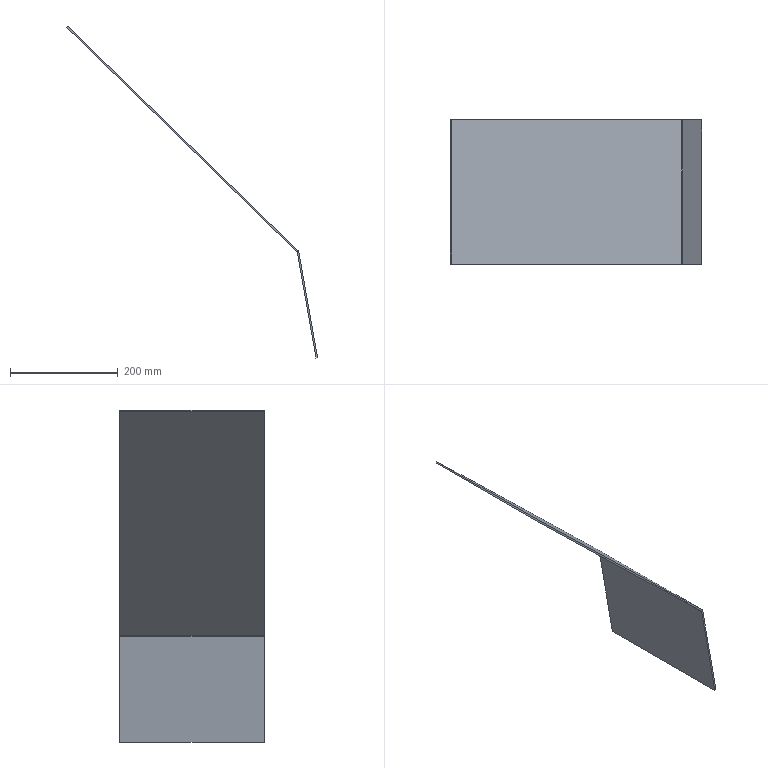Part | STEP file | floating channel bottom plate--2025.12.03 | 1 solid | 10 faces | box 466.015 x 268.5 x 616.159 mm | volume 643321 mm3 | plane 8 | cylinder 2 | commonest cylinder face diameters 6 x1 12 x1
STEP:
#1=CARTESIAN_POINT('',(0.,0.,0.));
#2=DIRECTION('',(0.,0.,1.));
#3=DIRECTION('',(1.,0.,0.));
#4=AXIS2_PLACEMENT_3D('',#1,#2,#3);
#5=CARTESIAN_POINT('',(1644.219,36.5,96.));
#6=VERTEX_POINT('',#5);
#7=CARTESIAN_POINT('',(2071.793,36.5,-320.384));
#8=VERTEX_POINT('',#7);
#9=CARTESIAN_POINT('',(1644.219,36.5,96.));
#10=DIRECTION('',(0.7164,0.,-0.6977));
#11=VECTOR('',#10,1.);
#12=LINE('',#9,#11);
#13=CARTESIAN_POINT('',(1644.219,305.,96.));
#14=DIRECTION('',(-0.6977,0.,-0.7164));
#15=DIRECTION('',(0.7164,0.,-0.6977));
#16=AXIS2_PLACEMENT_3D('',#13,#14,#15);
#17=PLANE('',#16);
#18=CARTESIAN_POINT('',(0.,268.5));
#19=DIRECTION('',(1.,0.));
#20=VECTOR('',#19,1.);
#21=LINE('',#18,#20);
#22=(GEOMETRIC_REPRESENTATION_CONTEXT(2)PARAMETRIC_REPRESENTATION_CONTEXT()REPRESENTATION_CONTEXT('',''));
#23=DEFINITIONAL_REPRESENTATION('',(#21),#22);
#24=PCURVE('',#17,#23);
#25=CARTESIAN_POINT('',(0.,36.5,0.));
#26=DIRECTION('',(0.,-1.,0.));
#27=DIRECTION('',(0.,0.,1.));
#28=AXIS2_PLACEMENT_3D('',#25,#26,#27);
#29=PLANE('',#28);
#30=CARTESIAN_POINT('',(96.,-1644.219));
#31=DIRECTION('',(-0.6977,-0.7164));
#32=VECTOR('',#31,1.);
#33=LINE('',#30,#32);
#34=(GEOMETRIC_REPRESENTATION_CONTEXT(2)PARAMETRIC_REPRESENTATION_CONTEXT()REPRESENTATION_CONTEXT('',''));
#35=DEFINITIONAL_REPRESENTATION('',(#33),#34);
#36=PCURVE('',#29,#35);
#37=SURFACE_CURVE('',#12,(#24,#36),.PCURVE_S1.);
#38=EDGE_CURVE('',#6,#8,#37,.T.);
#39=ORIENTED_EDGE('',*,*,#38,.T.);
#40=CARTESIAN_POINT('',(2071.793,305.,-320.384));
#41=VERTEX_POINT('',#40);
#42=CARTESIAN_POINT('',(2071.793,305.,-320.384));
#43=DIRECTION('',(0.,1.,0.));
#44=VECTOR('',#43,1.);
#45=LINE('',#42,#44);
#46=CARTESIAN_POINT('',(596.821,0.));
#47=DIRECTION('',(0.,-1.));
#48=VECTOR('',#47,1.);
#49=LINE('',#46,#48);
#50=(GEOMETRIC_REPRESENTATION_CONTEXT(2)PARAMETRIC_REPRESENTATION_CONTEXT()REPRESENTATION_CONTEXT('',''));
#51=DEFINITIONAL_REPRESENTATION('',(#49),#50);
#52=PCURVE('',#17,#51);
#53=CARTESIAN_POINT('',(2067.606,305.,-324.683));
#54=DIRECTION('',(0.,-1.,0.));
#55=DIRECTION('',(0.,0.,1.));
#56=AXIS2_PLACEMENT_3D('',#53,#54,#55);
#57=CYLINDRICAL_SURFACE('',#56,6.);
#58=CARTESIAN_POINT('',(5.511,0.));
#59=DIRECTION('',(0.,-1.));
#60=VECTOR('',#59,1.);
#61=LINE('',#58,#60);
#62=(GEOMETRIC_REPRESENTATION_CONTEXT(2)PARAMETRIC_REPRESENTATION_CONTEXT()REPRESENTATION_CONTEXT('',''));
#63=DEFINITIONAL_REPRESENTATION('',(#61),#62);
#64=PCURVE('',#57,#63);
#65=SURFACE_CURVE('',#45,(#52,#64),.PCURVE_S1.);
#66=EDGE_CURVE('',#8,#41,#65,.T.);
#67=ORIENTED_EDGE('',*,*,#66,.T.);
#68=CARTESIAN_POINT('',(1644.219,305.,96.));
#69=VERTEX_POINT('',#68);
#70=CARTESIAN_POINT('',(1644.219,305.,96.));
#71=DIRECTION('',(0.7164,0.,-0.6977));
#72=VECTOR('',#71,1.);
#73=LINE('',#70,#72);
#74=CARTESIAN_POINT('',(0.,0.));
#75=DIRECTION('',(1.,0.));
#76=VECTOR('',#75,1.);
#77=LINE('',#74,#76);
#78=(GEOMETRIC_REPRESENTATION_CONTEXT(2)PARAMETRIC_REPRESENTATION_CONTEXT()REPRESENTATION_CONTEXT('',''));
#79=DEFINITIONAL_REPRESENTATION('',(#77),#78);
#80=PCURVE('',#17,#79);
#81=CARTESIAN_POINT('',(0.,305.,0.));
#82=DIRECTION('',(0.,-1.,0.));
#83=DIRECTION('',(0.,0.,1.));
#84=AXIS2_PLACEMENT_3D('',#81,#82,#83);
#85=PLANE('',#84);
#86=CARTESIAN_POINT('',(96.,-1644.219));
#87=DIRECTION('',(-0.6977,-0.7164));
#88=VECTOR('',#87,1.);
#89=LINE('',#86,#88);
#90=(GEOMETRIC_REPRESENTATION_CONTEXT(2)PARAMETRIC_REPRESENTATION_CONTEXT()REPRESENTATION_CONTEXT('',''));
#91=DEFINITIONAL_REPRESENTATION('',(#89),#90);
#92=PCURVE('',#85,#91);
#93=SURFACE_CURVE('',#73,(#80,#92),.PCURVE_S1.);
#94=EDGE_CURVE('',#69,#41,#93,.T.);
#95=ORIENTED_EDGE('',*,*,#94,.F.);
#96=CARTESIAN_POINT('',(1644.219,305.,96.));
#97=DIRECTION('',(0.,-1.,0.));
#98=VECTOR('',#97,1.);
#99=LINE('',#96,#98);
#100=CARTESIAN_POINT('',(0.,0.));
#101=DIRECTION('',(0.,1.));
#102=VECTOR('',#101,1.);
#103=LINE('',#100,#102);
#104=(GEOMETRIC_REPRESENTATION_CONTEXT(2)PARAMETRIC_REPRESENTATION_CONTEXT()REPRESENTATION_CONTEXT('',''));
#105=DEFINITIONAL_REPRESENTATION('',(#103),#104);
#106=PCURVE('',#17,#105);
#107=CARTESIAN_POINT('',(1642.126,305.,93.851));
#108=DIRECTION('',(0.7164,0.,-0.6977));
#109=DIRECTION('',(0.6977,0.,0.7164));
#110=AXIS2_PLACEMENT_3D('',#107,#108,#109);
#111=PLANE('',#110);
#112=CARTESIAN_POINT('',(3.,0.));
#113=DIRECTION('',(0.,1.));
#114=VECTOR('',#113,1.);
#115=LINE('',#112,#114);
#116=(GEOMETRIC_REPRESENTATION_CONTEXT(2)PARAMETRIC_REPRESENTATION_CONTEXT()REPRESENTATION_CONTEXT('',''));
#117=DEFINITIONAL_REPRESENTATION('',(#115),#116);
#118=PCURVE('',#111,#117);
#119=SURFACE_CURVE('',#99,(#106,#118),.PCURVE_S1.);
#120=EDGE_CURVE('',#69,#6,#119,.T.);
#121=ORIENTED_EDGE('',*,*,#120,.T.);
#122=EDGE_LOOP('',(#39,#67,#95,#121));
#123=FACE_BOUND('',#122,.T.);
#124=ADVANCED_FACE('',(#123),#17,.F.);
#125=CARTESIAN_POINT('',(2073.515,305.,-323.639));
#126=VERTEX_POINT('',#125);
#127=CARTESIAN_POINT('',(2108.142,305.,-519.637));
#128=VERTEX_POINT('',#127);
#129=CARTESIAN_POINT('',(2073.178,305.,-321.734));
#130=DIRECTION('',(0.174,0.,-0.9848));
#131=VECTOR('',#130,1.);
#132=LINE('',#129,#131);
#133=CARTESIAN_POINT('',(2073.178,305.,-321.734));
#134=DIRECTION('',(-0.9848,0.,-0.174));
#135=DIRECTION('',(0.174,0.,-0.9848));
#136=AXIS2_PLACEMENT_3D('',#133,#134,#135);
#137=PLANE('',#136);
#138=CARTESIAN_POINT('',(0.,0.));
#139=DIRECTION('',(1.,0.));
#140=VECTOR('',#139,1.);
#141=LINE('',#138,#140);
#142=(GEOMETRIC_REPRESENTATION_CONTEXT(2)PARAMETRIC_REPRESENTATION_CONTEXT()REPRESENTATION_CONTEXT('',''));
#143=DEFINITIONAL_REPRESENTATION('',(#141),#142);
#144=PCURVE('',#137,#143);
#145=CARTESIAN_POINT('',(-321.734,-2073.178));
#146=DIRECTION('',(-0.9848,-0.174));
#147=VECTOR('',#146,1.);
#148=LINE('',#145,#147);
#149=(GEOMETRIC_REPRESENTATION_CONTEXT(2)PARAMETRIC_REPRESENTATION_CONTEXT()REPRESENTATION_CONTEXT('',''));
#150=DEFINITIONAL_REPRESENTATION('',(#148),#149);
#151=PCURVE('',#85,#150);
#152=SURFACE_CURVE('',#132,(#144,#151),.PCURVE_S1.);
#153=EDGE_CURVE('',#126,#128,#152,.T.);
#154=ORIENTED_EDGE('',*,*,#153,.F.);
#155=CARTESIAN_POINT('',(2073.515,36.5,-323.639));
#156=VERTEX_POINT('',#155);
#157=CARTESIAN_POINT('',(2073.515,305.,-323.639));
#158=DIRECTION('',(0.,-1.,0.));
#159=VECTOR('',#158,1.);
#160=LINE('',#157,#159);
#161=CARTESIAN_POINT('',(1.935,0.));
#162=DIRECTION('',(0.,1.));
#163=VECTOR('',#162,1.);
#164=LINE('',#161,#163);
#165=(GEOMETRIC_REPRESENTATION_CONTEXT(2)PARAMETRIC_REPRESENTATION_CONTEXT()REPRESENTATION_CONTEXT('',''));
#166=DEFINITIONAL_REPRESENTATION('',(#164),#165);
#167=PCURVE('',#137,#166);
#168=CARTESIAN_POINT('',(4.887,0.));
#169=DIRECTION('',(0.,1.));
#170=VECTOR('',#169,1.);
#171=LINE('',#168,#170);
#172=(GEOMETRIC_REPRESENTATION_CONTEXT(2)PARAMETRIC_REPRESENTATION_CONTEXT()REPRESENTATION_CONTEXT('',''));
#173=DEFINITIONAL_REPRESENTATION('',(#171),#172);
#174=PCURVE('',#57,#173);
#175=SURFACE_CURVE('',#160,(#167,#174),.PCURVE_S1.);
#176=EDGE_CURVE('',#126,#156,#175,.T.);
#177=ORIENTED_EDGE('',*,*,#176,.T.);
#178=CARTESIAN_POINT('',(2108.142,36.5,-519.637));
#179=VERTEX_POINT('',#178);
#180=CARTESIAN_POINT('',(2073.178,36.5,-321.734));
#181=DIRECTION('',(0.174,0.,-0.9848));
#182=VECTOR('',#181,1.);
#183=LINE('',#180,#182);
#184=CARTESIAN_POINT('',(0.,268.5));
#185=DIRECTION('',(1.,0.));
#186=VECTOR('',#185,1.);
#187=LINE('',#184,#186);
#188=(GEOMETRIC_REPRESENTATION_CONTEXT(2)PARAMETRIC_REPRESENTATION_CONTEXT()REPRESENTATION_CONTEXT('',''));
#189=DEFINITIONAL_REPRESENTATION('',(#187),#188);
#190=PCURVE('',#137,#189);
#191=CARTESIAN_POINT('',(-321.734,-2073.178));
#192=DIRECTION('',(-0.9848,-0.174));
#193=VECTOR('',#192,1.);
#194=LINE('',#191,#193);
#195=(GEOMETRIC_REPRESENTATION_CONTEXT(2)PARAMETRIC_REPRESENTATION_CONTEXT()REPRESENTATION_CONTEXT('',''));
#196=DEFINITIONAL_REPRESENTATION('',(#194),#195);
#197=PCURVE('',#29,#196);
#198=SURFACE_CURVE('',#183,(#190,#197),.PCURVE_S1.);
#199=EDGE_CURVE('',#156,#179,#198,.T.);
#200=ORIENTED_EDGE('',*,*,#199,.T.);
#201=CARTESIAN_POINT('',(2108.142,305.,-519.637));
#202=DIRECTION('',(0.,-1.,0.));
#203=VECTOR('',#202,1.);
#204=LINE('',#201,#203);
#205=CARTESIAN_POINT('',(200.967,0.));
#206=DIRECTION('',(0.,1.));
#207=VECTOR('',#206,1.);
#208=LINE('',#205,#207);
#209=(GEOMETRIC_REPRESENTATION_CONTEXT(2)PARAMETRIC_REPRESENTATION_CONTEXT()REPRESENTATION_CONTEXT('',''));
#210=DEFINITIONAL_REPRESENTATION('',(#208),#209);
#211=PCURVE('',#137,#210);
#212=CARTESIAN_POINT('',(2108.142,305.,-519.637));
#213=DIRECTION('',(-0.174,0.,0.9848));
#214=DIRECTION('',(-0.9848,0.,-0.174));
#215=AXIS2_PLACEMENT_3D('',#212,#213,#214);
#216=PLANE('',#215);
#217=CARTESIAN_POINT('',(0.,0.));
#218=DIRECTION('',(0.,1.));
#219=VECTOR('',#218,1.);
#220=LINE('',#217,#219);
#221=(GEOMETRIC_REPRESENTATION_CONTEXT(2)PARAMETRIC_REPRESENTATION_CONTEXT()REPRESENTATION_CONTEXT('',''));
#222=DEFINITIONAL_REPRESENTATION('',(#220),#221);
#223=PCURVE('',#216,#222);
#224=SURFACE_CURVE('',#204,(#211,#223),.PCURVE_S1.);
#225=EDGE_CURVE('',#128,#179,#224,.T.);
#226=ORIENTED_EDGE('',*,*,#225,.F.);
#227=EDGE_LOOP('',(#154,#177,#200,#226));
#228=FACE_BOUND('',#227,.T.);
#229=ADVANCED_FACE('',(#228),#137,.F.);
#230=CARTESIAN_POINT('',(2105.187,36.5,-520.159));
#231=VERTEX_POINT('',#230);
#232=CARTESIAN_POINT('',(2108.142,36.5,-519.637));
#233=DIRECTION('',(-0.9848,0.,-0.174));
#234=VECTOR('',#233,1.);
#235=LINE('',#232,#234);
#236=CARTESIAN_POINT('',(0.,268.5));
#237=DIRECTION('',(1.,0.));
#238=VECTOR('',#237,1.);
#239=LINE('',#236,#238);
#240=(GEOMETRIC_REPRESENTATION_CONTEXT(2)PARAMETRIC_REPRESENTATION_CONTEXT()REPRESENTATION_CONTEXT('',''));
#241=DEFINITIONAL_REPRESENTATION('',(#239),#240);
#242=PCURVE('',#216,#241);
#243=CARTESIAN_POINT('',(-519.637,-2108.142));
#244=DIRECTION('',(-0.174,0.9848));
#245=VECTOR('',#244,1.);
#246=LINE('',#243,#245);
#247=(GEOMETRIC_REPRESENTATION_CONTEXT(2)PARAMETRIC_REPRESENTATION_CONTEXT()REPRESENTATION_CONTEXT('',''));
#248=DEFINITIONAL_REPRESENTATION('',(#246),#247);
#249=PCURVE('',#29,#248);
#250=SURFACE_CURVE('',#235,(#242,#249),.PCURVE_S1.);
#251=EDGE_CURVE('',#179,#231,#250,.T.);
#252=ORIENTED_EDGE('',*,*,#251,.T.);
#253=CARTESIAN_POINT('',(2105.187,305.,-520.159));
#254=VERTEX_POINT('',#253);
#255=CARTESIAN_POINT('',(2105.187,305.,-520.159));
#256=DIRECTION('',(0.,-1.,0.));
#257=VECTOR('',#256,1.);
#258=LINE('',#255,#257);
#259=CARTESIAN_POINT('',(3.,0.));
#260=DIRECTION('',(0.,1.));
#261=VECTOR('',#260,1.);
#262=LINE('',#259,#261);
#263=(GEOMETRIC_REPRESENTATION_CONTEXT(2)PARAMETRIC_REPRESENTATION_CONTEXT()REPRESENTATION_CONTEXT('',''));
#264=DEFINITIONAL_REPRESENTATION('',(#262),#263);
#265=PCURVE('',#216,#264);
#266=CARTESIAN_POINT('',(2105.187,305.,-520.159));
#267=DIRECTION('',(0.9848,0.,0.174));
#268=DIRECTION('',(-0.174,0.,0.9848));
#269=AXIS2_PLACEMENT_3D('',#266,#267,#268);
#270=PLANE('',#269);
#271=CARTESIAN_POINT('',(0.,0.));
#272=DIRECTION('',(0.,1.));
#273=VECTOR('',#272,1.);
#274=LINE('',#271,#273);
#275=(GEOMETRIC_REPRESENTATION_CONTEXT(2)PARAMETRIC_REPRESENTATION_CONTEXT()REPRESENTATION_CONTEXT('',''));
#276=DEFINITIONAL_REPRESENTATION('',(#274),#275);
#277=PCURVE('',#270,#276);
#278=SURFACE_CURVE('',#258,(#265,#277),.PCURVE_S1.);
#279=EDGE_CURVE('',#254,#231,#278,.T.);
#280=ORIENTED_EDGE('',*,*,#279,.F.);
#281=CARTESIAN_POINT('',(2108.142,305.,-519.637));
#282=DIRECTION('',(-0.9848,0.,-0.174));
#283=VECTOR('',#282,1.);
#284=LINE('',#281,#283);
#285=CARTESIAN_POINT('',(0.,0.));
#286=DIRECTION('',(1.,0.));
#287=VECTOR('',#286,1.);
#288=LINE('',#285,#287);
#289=(GEOMETRIC_REPRESENTATION_CONTEXT(2)PARAMETRIC_REPRESENTATION_CONTEXT()REPRESENTATION_CONTEXT('',''));
#290=DEFINITIONAL_REPRESENTATION('',(#288),#289);
#291=PCURVE('',#216,#290);
#292=CARTESIAN_POINT('',(-519.637,-2108.142));
#293=DIRECTION('',(-0.174,0.9848));
#294=VECTOR('',#293,1.);
#295=LINE('',#292,#294);
#296=(GEOMETRIC_REPRESENTATION_CONTEXT(2)PARAMETRIC_REPRESENTATION_CONTEXT()REPRESENTATION_CONTEXT('',''));
#297=DEFINITIONAL_REPRESENTATION('',(#295),#296);
#298=PCURVE('',#85,#297);
#299=SURFACE_CURVE('',#284,(#291,#298),.PCURVE_S1.);
#300=EDGE_CURVE('',#128,#254,#299,.T.);
#301=ORIENTED_EDGE('',*,*,#300,.F.);
#302=ORIENTED_EDGE('',*,*,#225,.T.);
#303=EDGE_LOOP('',(#252,#280,#301,#302));
#304=FACE_BOUND('',#303,.T.);
#305=ADVANCED_FACE('',(#304),#216,.F.);
#306=CARTESIAN_POINT('',(2070.561,36.5,-324.161));
#307=VERTEX_POINT('',#306);
#308=CARTESIAN_POINT('',(2105.187,36.5,-520.159));
#309=DIRECTION('',(-0.174,0.,0.9848));
#310=VECTOR('',#309,1.);
#311=LINE('',#308,#310);
#312=CARTESIAN_POINT('',(0.,268.5));
#313=DIRECTION('',(1.,0.));
#314=VECTOR('',#313,1.);
#315=LINE('',#312,#314);
#316=(GEOMETRIC_REPRESENTATION_CONTEXT(2)PARAMETRIC_REPRESENTATION_CONTEXT()REPRESENTATION_CONTEXT('',''));
#317=DEFINITIONAL_REPRESENTATION('',(#315),#316);
#318=PCURVE('',#270,#317);
#319=CARTESIAN_POINT('',(-520.159,-2105.187));
#320=DIRECTION('',(0.9848,0.174));
#321=VECTOR('',#320,1.);
#322=LINE('',#319,#321);
#323=(GEOMETRIC_REPRESENTATION_CONTEXT(2)PARAMETRIC_REPRESENTATION_CONTEXT()REPRESENTATION_CONTEXT('',''));
#324=DEFINITIONAL_REPRESENTATION('',(#322),#323);
#325=PCURVE('',#29,#324);
#326=SURFACE_CURVE('',#311,(#318,#325),.PCURVE_S1.);
#327=EDGE_CURVE('',#231,#307,#326,.T.);
#328=ORIENTED_EDGE('',*,*,#327,.T.);
#329=CARTESIAN_POINT('',(2070.561,305.,-324.161));
#330=VERTEX_POINT('',#329);
#331=CARTESIAN_POINT('',(2070.561,305.,-324.161));
#332=DIRECTION('',(0.,1.,0.));
#333=VECTOR('',#332,1.);
#334=LINE('',#331,#333);
#335=CARTESIAN_POINT('',(199.033,0.));
#336=DIRECTION('',(0.,-1.));
#337=VECTOR('',#336,1.);
#338=LINE('',#335,#337);
#339=(GEOMETRIC_REPRESENTATION_CONTEXT(2)PARAMETRIC_REPRESENTATION_CONTEXT()REPRESENTATION_CONTEXT('',''));
#340=DEFINITIONAL_REPRESENTATION('',(#338),#339);
#341=PCURVE('',#270,#340);
#342=CARTESIAN_POINT('',(2067.606,305.,-324.683));
#343=DIRECTION('',(0.,1.,0.));
#344=DIRECTION('',(0.,0.,-1.));
#345=AXIS2_PLACEMENT_3D('',#342,#343,#344);
#346=CYLINDRICAL_SURFACE('',#345,3.);
#347=CARTESIAN_POINT('',(4.538,0.));
#348=DIRECTION('',(0.,1.));
#349=VECTOR('',#348,1.);
#350=LINE('',#347,#349);
#351=(GEOMETRIC_REPRESENTATION_CONTEXT(2)PARAMETRIC_REPRESENTATION_CONTEXT()REPRESENTATION_CONTEXT('',''));
#352=DEFINITIONAL_REPRESENTATION('',(#350),#351);
#353=PCURVE('',#346,#352);
#354=SURFACE_CURVE('',#334,(#341,#353),.PCURVE_S1.);
#355=EDGE_CURVE('',#307,#330,#354,.T.);
#356=ORIENTED_EDGE('',*,*,#355,.T.);
#357=CARTESIAN_POINT('',(2105.187,305.,-520.159));
#358=DIRECTION('',(-0.174,0.,0.9848));
#359=VECTOR('',#358,1.);
#360=LINE('',#357,#359);
#361=CARTESIAN_POINT('',(0.,0.));
#362=DIRECTION('',(1.,0.));
#363=VECTOR('',#362,1.);
#364=LINE('',#361,#363);
#365=(GEOMETRIC_REPRESENTATION_CONTEXT(2)PARAMETRIC_REPRESENTATION_CONTEXT()REPRESENTATION_CONTEXT('',''));
#366=DEFINITIONAL_REPRESENTATION('',(#364),#365);
#367=PCURVE('',#270,#366);
#368=CARTESIAN_POINT('',(-520.159,-2105.187));
#369=DIRECTION('',(0.9848,0.174));
#370=VECTOR('',#369,1.);
#371=LINE('',#368,#370);
#372=(GEOMETRIC_REPRESENTATION_CONTEXT(2)PARAMETRIC_REPRESENTATION_CONTEXT()REPRESENTATION_CONTEXT('',''));
#373=DEFINITIONAL_REPRESENTATION('',(#371),#372);
#374=PCURVE('',#85,#373);
#375=SURFACE_CURVE('',#360,(#367,#374),.PCURVE_S1.);
#376=EDGE_CURVE('',#254,#330,#375,.T.);
#377=ORIENTED_EDGE('',*,*,#376,.F.);
#378=ORIENTED_EDGE('',*,*,#279,.T.);
#379=EDGE_LOOP('',(#328,#356,#377,#378));
#380=FACE_BOUND('',#379,.T.);
#381=ADVANCED_FACE('',(#380),#270,.F.);
#382=CARTESIAN_POINT('',(2069.699,305.,-322.534));
#383=VERTEX_POINT('',#382);
#384=CARTESIAN_POINT('',(1642.126,305.,93.851));
#385=VERTEX_POINT('',#384);
#386=CARTESIAN_POINT('',(2070.392,305.,-323.209));
#387=DIRECTION('',(-0.7164,0.,0.6977));
#388=VECTOR('',#387,1.);
#389=LINE('',#386,#388);
#390=CARTESIAN_POINT('',(2070.392,305.,-323.209));
#391=DIRECTION('',(0.6977,0.,0.7164));
#392=DIRECTION('',(-0.7164,0.,0.6977));
#393=AXIS2_PLACEMENT_3D('',#390,#391,#392);
#394=PLANE('',#393);
#395=CARTESIAN_POINT('',(0.,0.));
#396=DIRECTION('',(1.,0.));
#397=VECTOR('',#396,1.);
#398=LINE('',#395,#397);
#399=(GEOMETRIC_REPRESENTATION_CONTEXT(2)PARAMETRIC_REPRESENTATION_CONTEXT()REPRESENTATION_CONTEXT('',''));
#400=DEFINITIONAL_REPRESENTATION('',(#398),#399);
#401=PCURVE('',#394,#400);
#402=CARTESIAN_POINT('',(-323.209,-2070.392));
#403=DIRECTION('',(0.6977,0.7164));
#404=VECTOR('',#403,1.);
#405=LINE('',#402,#404);
#406=(GEOMETRIC_REPRESENTATION_CONTEXT(2)PARAMETRIC_REPRESENTATION_CONTEXT()REPRESENTATION_CONTEXT('',''));
#407=DEFINITIONAL_REPRESENTATION('',(#405),#406);
#408=PCURVE('',#85,#407);
#409=SURFACE_CURVE('',#389,(#401,#408),.PCURVE_S1.);
#410=EDGE_CURVE('',#383,#385,#409,.T.);
#411=ORIENTED_EDGE('',*,*,#410,.F.);
#412=CARTESIAN_POINT('',(2069.699,36.5,-322.534));
#413=VERTEX_POINT('',#412);
#414=CARTESIAN_POINT('',(2069.699,36.5,-322.534));
#415=DIRECTION('',(0.,-1.,0.));
#416=VECTOR('',#415,1.);
#417=LINE('',#414,#416);
#418=CARTESIAN_POINT('',(0.9673,268.5));
#419=DIRECTION('',(0.,1.));
#420=VECTOR('',#419,1.);
#421=LINE('',#418,#420);
#422=(GEOMETRIC_REPRESENTATION_CONTEXT(2)PARAMETRIC_REPRESENTATION_CONTEXT()REPRESENTATION_CONTEXT('',''));
#423=DEFINITIONAL_REPRESENTATION('',(#421),#422);
#424=PCURVE('',#394,#423);
#425=CARTESIAN_POINT('',(3.914,-268.5));
#426=DIRECTION('',(0.,-1.));
#427=VECTOR('',#426,1.);
#428=LINE('',#425,#427);
#429=(GEOMETRIC_REPRESENTATION_CONTEXT(2)PARAMETRIC_REPRESENTATION_CONTEXT()REPRESENTATION_CONTEXT('',''));
#430=DEFINITIONAL_REPRESENTATION('',(#428),#429);
#431=PCURVE('',#346,#430);
#432=SURFACE_CURVE('',#417,(#424,#431),.PCURVE_S1.);
#433=EDGE_CURVE('',#383,#413,#432,.T.);
#434=ORIENTED_EDGE('',*,*,#433,.T.);
#435=CARTESIAN_POINT('',(1642.126,36.5,93.851));
#436=VERTEX_POINT('',#435);
#437=CARTESIAN_POINT('',(2070.392,36.5,-323.209));
#438=DIRECTION('',(-0.7164,0.,0.6977));
#439=VECTOR('',#438,1.);
#440=LINE('',#437,#439);
#441=CARTESIAN_POINT('',(0.,268.5));
#442=DIRECTION('',(1.,0.));
#443=VECTOR('',#442,1.);
#444=LINE('',#441,#443);
#445=(GEOMETRIC_REPRESENTATION_CONTEXT(2)PARAMETRIC_REPRESENTATION_CONTEXT()REPRESENTATION_CONTEXT('',''));
#446=DEFINITIONAL_REPRESENTATION('',(#444),#445);
#447=PCURVE('',#394,#446);
#448=CARTESIAN_POINT('',(-323.209,-2070.392));
#449=DIRECTION('',(0.6977,0.7164));
#450=VECTOR('',#449,1.);
#451=LINE('',#448,#450);
#452=(GEOMETRIC_REPRESENTATION_CONTEXT(2)PARAMETRIC_REPRESENTATION_CONTEXT()REPRESENTATION_CONTEXT('',''));
#453=DEFINITIONAL_REPRESENTATION('',(#451),#452);
#454=PCURVE('',#29,#453);
#455=SURFACE_CURVE('',#440,(#447,#454),.PCURVE_S1.);
#456=EDGE_CURVE('',#413,#436,#455,.T.);
#457=ORIENTED_EDGE('',*,*,#456,.T.);
#458=CARTESIAN_POINT('',(1642.126,305.,93.851));
#459=DIRECTION('',(0.,-1.,0.));
#460=VECTOR('',#459,1.);
#461=LINE('',#458,#460);
#462=CARTESIAN_POINT('',(597.788,0.));
#463=DIRECTION('',(0.,1.));
#464=VECTOR('',#463,1.);
#465=LINE('',#462,#464);
#466=(GEOMETRIC_REPRESENTATION_CONTEXT(2)PARAMETRIC_REPRESENTATION_CONTEXT()REPRESENTATION_CONTEXT('',''));
#467=DEFINITIONAL_REPRESENTATION('',(#465),#466);
#468=PCURVE('',#394,#467);
#469=CARTESIAN_POINT('',(0.,0.));
#470=DIRECTION('',(0.,1.));
#471=VECTOR('',#470,1.);
#472=LINE('',#469,#471);
#473=(GEOMETRIC_REPRESENTATION_CONTEXT(2)PARAMETRIC_REPRESENTATION_CONTEXT()REPRESENTATION_CONTEXT('',''));
#474=DEFINITIONAL_REPRESENTATION('',(#472),#473);
#475=PCURVE('',#111,#474);
#476=SURFACE_CURVE('',#461,(#468,#475),.PCURVE_S1.);
#477=EDGE_CURVE('',#385,#436,#476,.T.);
#478=ORIENTED_EDGE('',*,*,#477,.F.);
#479=EDGE_LOOP('',(#411,#434,#457,#478));
#480=FACE_BOUND('',#479,.T.);
#481=ADVANCED_FACE('',(#480),#394,.F.);
#482=CARTESIAN_POINT('',(1642.126,36.5,93.851));
#483=DIRECTION('',(0.6977,0.,0.7164));
#484=VECTOR('',#483,1.);
#485=LINE('',#482,#484);
#486=CARTESIAN_POINT('',(0.,268.5));
#487=DIRECTION('',(1.,0.));
#488=VECTOR('',#487,1.);
#489=LINE('',#486,#488);
#490=(GEOMETRIC_REPRESENTATION_CONTEXT(2)PARAMETRIC_REPRESENTATION_CONTEXT()REPRESENTATION_CONTEXT('',''));
#491=DEFINITIONAL_REPRESENTATION('',(#489),#490);
#492=PCURVE('',#111,#491);
#493=CARTESIAN_POINT('',(93.851,-1642.126));
#494=DIRECTION('',(0.7164,-0.6977));
#495=VECTOR('',#494,1.);
#496=LINE('',#493,#495);
#497=(GEOMETRIC_REPRESENTATION_CONTEXT(2)PARAMETRIC_REPRESENTATION_CONTEXT()REPRESENTATION_CONTEXT('',''));
#498=DEFINITIONAL_REPRESENTATION('',(#496),#497);
#499=PCURVE('',#29,#498);
#500=SURFACE_CURVE('',#485,(#492,#499),.PCURVE_S1.);
#501=EDGE_CURVE('',#436,#6,#500,.T.);
#502=ORIENTED_EDGE('',*,*,#501,.T.);
#503=ORIENTED_EDGE('',*,*,#120,.F.);
#504=CARTESIAN_POINT('',(1642.126,305.,93.851));
#505=DIRECTION('',(0.6977,0.,0.7164));
#506=VECTOR('',#505,1.);
#507=LINE('',#504,#506);
#508=CARTESIAN_POINT('',(0.,0.));
#509=DIRECTION('',(1.,0.));
#510=VECTOR('',#509,1.);
#511=LINE('',#508,#510);
#512=(GEOMETRIC_REPRESENTATION_CONTEXT(2)PARAMETRIC_REPRESENTATION_CONTEXT()REPRESENTATION_CONTEXT('',''));
#513=DEFINITIONAL_REPRESENTATION('',(#511),#512);
#514=PCURVE('',#111,#513);
#515=CARTESIAN_POINT('',(93.851,-1642.126));
#516=DIRECTION('',(0.7164,-0.6977));
#517=VECTOR('',#516,1.);
#518=LINE('',#515,#517);
#519=(GEOMETRIC_REPRESENTATION_CONTEXT(2)PARAMETRIC_REPRESENTATION_CONTEXT()REPRESENTATION_CONTEXT('',''));
#520=DEFINITIONAL_REPRESENTATION('',(#518),#519);
#521=PCURVE('',#85,#520);
#522=SURFACE_CURVE('',#507,(#514,#521),.PCURVE_S1.);
#523=EDGE_CURVE('',#385,#69,#522,.T.);
#524=ORIENTED_EDGE('',*,*,#523,.F.);
#525=ORIENTED_EDGE('',*,*,#477,.T.);
#526=EDGE_LOOP('',(#502,#503,#524,#525));
#527=FACE_BOUND('',#526,.T.);
#528=ADVANCED_FACE('',(#527),#111,.F.);
#529=ORIENTED_EDGE('',*,*,#94,.T.);
#530=CARTESIAN_POINT('',(2067.606,305.,-324.683));
#531=DIRECTION('',(0.,1.,0.));
#532=DIRECTION('',(0.,0.,-1.));
#533=AXIS2_PLACEMENT_3D('',#530,#531,#532);
#534=CIRCLE('',#533,6.);
#535=CARTESIAN_POINT('',(-330.683,-2067.606));
#536=CARTESIAN_POINT('',(-330.683,-2057.214));
#537=CARTESIAN_POINT('',(-321.683,-2062.41));
#538=CARTESIAN_POINT('',(-312.683,-2067.606));
#539=CARTESIAN_POINT('',(-321.683,-2072.803));
#540=CARTESIAN_POINT('',(-330.683,-2077.999));
#541=CARTESIAN_POINT('',(-330.683,-2067.606));
#542=(BOUNDED_CURVE()B_SPLINE_CURVE(2,(#535,#536,#537,#538,#539,#540,#541),.UNSPECIFIED.,.T.,.F.)B_SPLINE_CURVE_WITH_KNOTS((1,2,2,2,2,1),(-2.094,0.,2.094,4.189,6.283,8.378),.UNSPECIFIED.)CURVE()GEOMETRIC_REPRESENTATION_ITEM()RATIONAL_B_SPLINE_CURVE((1.,0.5,1.,0.5,1.,0.5,1.))REPRESENTATION_ITEM(''));
#543=(GEOMETRIC_REPRESENTATION_CONTEXT(2)PARAMETRIC_REPRESENTATION_CONTEXT()REPRESENTATION_CONTEXT('',''));
#544=DEFINITIONAL_REPRESENTATION('',(#542),#543);
#545=PCURVE('',#85,#544);
#546=CARTESIAN_POINT('',(9.425,0.));
#547=DIRECTION('',(-1.,0.));
#548=VECTOR('',#547,1.);
#549=LINE('',#546,#548);
#550=(GEOMETRIC_REPRESENTATION_CONTEXT(2)PARAMETRIC_REPRESENTATION_CONTEXT()REPRESENTATION_CONTEXT('',''));
#551=DEFINITIONAL_REPRESENTATION('',(#549),#550);
#552=PCURVE('',#57,#551);
#553=SURFACE_CURVE('',#534,(#545,#552),.PCURVE_S1.);
#554=EDGE_CURVE('',#41,#126,#553,.T.);
#555=ORIENTED_EDGE('',*,*,#554,.T.);
#556=ORIENTED_EDGE('',*,*,#153,.T.);
#557=ORIENTED_EDGE('',*,*,#300,.T.);
#558=ORIENTED_EDGE('',*,*,#376,.T.);
#559=CARTESIAN_POINT('',(2067.606,305.,-324.683));
#560=DIRECTION('',(0.,-1.,0.));
#561=DIRECTION('',(0.,0.,-1.));
#562=AXIS2_PLACEMENT_3D('',#559,#560,#561);
#563=CIRCLE('',#562,3.);
#564=CARTESIAN_POINT('',(-324.683,-2067.606));
#565=DIRECTION('',(-1.,0.));
#566=AXIS2_PLACEMENT_2D('',#564,#565);
#567=CIRCLE('',#566,3.);
#568=(GEOMETRIC_REPRESENTATION_CONTEXT(2)PARAMETRIC_REPRESENTATION_CONTEXT()REPRESENTATION_CONTEXT('',''));
#569=DEFINITIONAL_REPRESENTATION('',(#567),#568);
#570=PCURVE('',#85,#569);
#571=CARTESIAN_POINT('',(6.283,0.));
#572=DIRECTION('',(-1.,0.));
#573=VECTOR('',#572,1.);
#574=LINE('',#571,#573);
#575=(GEOMETRIC_REPRESENTATION_CONTEXT(2)PARAMETRIC_REPRESENTATION_CONTEXT()REPRESENTATION_CONTEXT('',''));
#576=DEFINITIONAL_REPRESENTATION('',(#574),#575);
#577=PCURVE('',#346,#576);
#578=SURFACE_CURVE('',#563,(#570,#577),.PCURVE_S1.);
#579=EDGE_CURVE('',#330,#383,#578,.T.);
#580=ORIENTED_EDGE('',*,*,#579,.T.);
#581=ORIENTED_EDGE('',*,*,#410,.T.);
#582=ORIENTED_EDGE('',*,*,#523,.T.);
#583=EDGE_LOOP('',(#529,#555,#556,#557,#558,#580,#581,#582));
#584=FACE_BOUND('',#583,.T.);
#585=ADVANCED_FACE('',(#584),#85,.F.);
#586=ORIENTED_EDGE('',*,*,#199,.F.);
#587=CARTESIAN_POINT('',(2067.606,36.5,-324.683));
#588=DIRECTION('',(0.,-1.,0.));
#589=DIRECTION('',(0.,0.,-1.));
#590=AXIS2_PLACEMENT_3D('',#587,#588,#589);
#591=CIRCLE('',#590,6.);
#592=CARTESIAN_POINT('',(-324.683,-2067.606));
#593=DIRECTION('',(-1.,0.));
#594=AXIS2_PLACEMENT_2D('',#592,#593);
#595=CIRCLE('',#594,6.);
#596=(GEOMETRIC_REPRESENTATION_CONTEXT(2)PARAMETRIC_REPRESENTATION_CONTEXT()REPRESENTATION_CONTEXT('',''));
#597=DEFINITIONAL_REPRESENTATION('',(#595),#596);
#598=PCURVE('',#29,#597);
#599=CARTESIAN_POINT('',(3.142,268.5));
#600=DIRECTION('',(1.,0.));
#601=VECTOR('',#600,1.);
#602=LINE('',#599,#601);
#603=(GEOMETRIC_REPRESENTATION_CONTEXT(2)PARAMETRIC_REPRESENTATION_CONTEXT()REPRESENTATION_CONTEXT('',''));
#604=DEFINITIONAL_REPRESENTATION('',(#602),#603);
#605=PCURVE('',#57,#604);
#606=SURFACE_CURVE('',#591,(#598,#605),.PCURVE_S1.);
#607=EDGE_CURVE('',#156,#8,#606,.T.);
#608=ORIENTED_EDGE('',*,*,#607,.T.);
#609=ORIENTED_EDGE('',*,*,#38,.F.);
#610=ORIENTED_EDGE('',*,*,#501,.F.);
#611=ORIENTED_EDGE('',*,*,#456,.F.);
#612=CARTESIAN_POINT('',(2067.606,36.5,-324.683));
#613=DIRECTION('',(0.,1.,0.));
#614=DIRECTION('',(0.,0.,-1.));
#615=AXIS2_PLACEMENT_3D('',#612,#613,#614);
#616=CIRCLE('',#615,3.);
#617=CARTESIAN_POINT('',(-327.683,-2067.606));
#618=CARTESIAN_POINT('',(-327.683,-2062.41));
#619=CARTESIAN_POINT('',(-323.183,-2065.008));
#620=CARTESIAN_POINT('',(-318.683,-2067.606));
#621=CARTESIAN_POINT('',(-323.183,-2070.205));
#622=CARTESIAN_POINT('',(-327.683,-2072.803));
#623=CARTESIAN_POINT('',(-327.683,-2067.606));
#624=(BOUNDED_CURVE()B_SPLINE_CURVE(2,(#617,#618,#619,#620,#621,#622,#623),.UNSPECIFIED.,.T.,.F.)B_SPLINE_CURVE_WITH_KNOTS((1,2,2,2,2,1),(-2.094,0.,2.094,4.189,6.283,8.378),.UNSPECIFIED.)CURVE()GEOMETRIC_REPRESENTATION_ITEM()RATIONAL_B_SPLINE_CURVE((1.,0.5,1.,0.5,1.,0.5,1.))REPRESENTATION_ITEM(''));
#625=(GEOMETRIC_REPRESENTATION_CONTEXT(2)PARAMETRIC_REPRESENTATION_CONTEXT()REPRESENTATION_CONTEXT('',''));
#626=DEFINITIONAL_REPRESENTATION('',(#624),#625);
#627=PCURVE('',#29,#626);
#628=CARTESIAN_POINT('',(0.,-268.5));
#629=DIRECTION('',(1.,0.));
#630=VECTOR('',#629,1.);
#631=LINE('',#628,#630);
#632=(GEOMETRIC_REPRESENTATION_CONTEXT(2)PARAMETRIC_REPRESENTATION_CONTEXT()REPRESENTATION_CONTEXT('',''));
#633=DEFINITIONAL_REPRESENTATION('',(#631),#632);
#634=PCURVE('',#346,#633);
#635=SURFACE_CURVE('',#616,(#627,#634),.PCURVE_S1.);
#636=EDGE_CURVE('',#413,#307,#635,.T.);
#637=ORIENTED_EDGE('',*,*,#636,.T.);
#638=ORIENTED_EDGE('',*,*,#327,.F.);
#639=ORIENTED_EDGE('',*,*,#251,.F.);
#640=EDGE_LOOP('',(#586,#608,#609,#610,#611,#637,#638,#639));
#641=FACE_BOUND('',#640,.T.);
#642=ADVANCED_FACE('',(#641),#29,.T.);
#643=ORIENTED_EDGE('',*,*,#433,.T.);
#644=ORIENTED_EDGE('',*,*,#636,.T.);
#645=ORIENTED_EDGE('',*,*,#355,.T.);
#646=ORIENTED_EDGE('',*,*,#579,.T.);
#647=EDGE_LOOP('',(#643,#644,#645,#646));
#648=FACE_BOUND('',#647,.F.);
#649=ADVANCED_FACE('',(#648),#346,.F.);
#650=ORIENTED_EDGE('',*,*,#554,.F.);
#651=ORIENTED_EDGE('',*,*,#66,.F.);
#652=ORIENTED_EDGE('',*,*,#607,.F.);
#653=ORIENTED_EDGE('',*,*,#176,.F.);
#654=EDGE_LOOP('',(#650,#651,#652,#653));
#655=FACE_BOUND('',#654,.T.);
#656=ADVANCED_FACE('',(#655),#57,.T.);
#657=CLOSED_SHELL('',(#124,#229,#305,#381,#481,#528,#585,#642,#649,#656));
#658=MANIFOLD_SOLID_BREP('',#657);
#659=(LENGTH_UNIT()NAMED_UNIT(*)SI_UNIT(.MILLI.,.METRE.));
#660=UNCERTAINTY_MEASURE_WITH_UNIT(LENGTH_MEASURE(0.0000001),#659,'','');
#661=(NAMED_UNIT(*)PLANE_ANGLE_UNIT()SI_UNIT($,.RADIAN.));
#662=(NAMED_UNIT(*)SI_UNIT($,.STERADIAN.)SOLID_ANGLE_UNIT());
#663=(GEOMETRIC_REPRESENTATION_CONTEXT(3)GLOBAL_UNCERTAINTY_ASSIGNED_CONTEXT((#660))GLOBAL_UNIT_ASSIGNED_CONTEXT((#659,#661,#662))REPRESENTATION_CONTEXT('',''));
#664=ADVANCED_BREP_SHAPE_REPRESENTATION('',(#4,#658),#663);